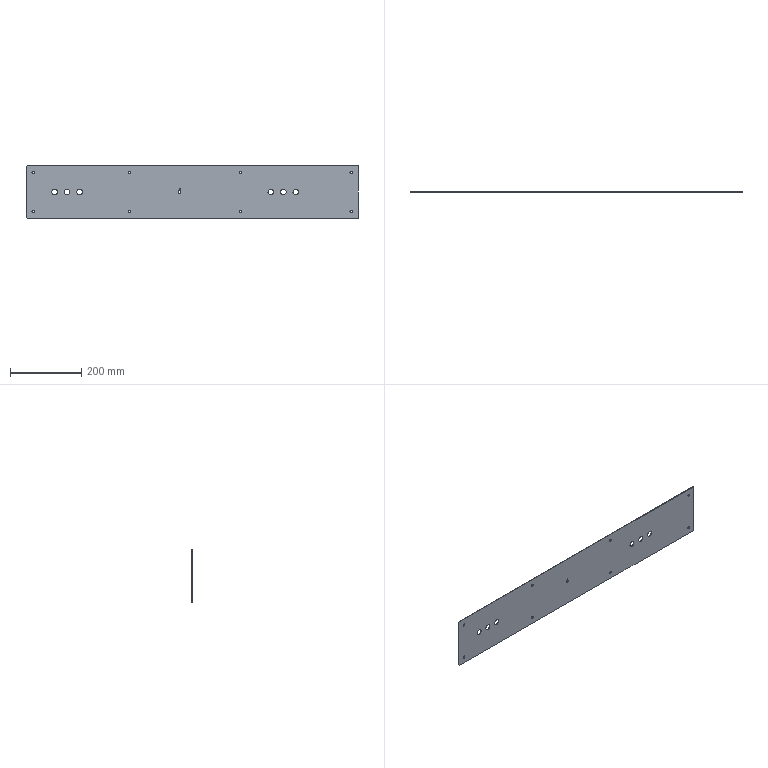Part | NX | 1 solid | 42 faces | box 929 x 2 x 150 mm | volume 275554 mm3 | cylinder 32 | plane 10 | commonest cylinder face diameters 7 x18 16 x12 3 x2
STEP:
#1=CARTESIAN_POINT('',(1280.5,-128.5,192.5));
#2=VERTEX_POINT('',#1);
#3=CARTESIAN_POINT('',(1287.5,-128.5,192.5));
#4=VERTEX_POINT('',#3);
#5=CARTESIAN_POINT('',(1284.,-128.5,192.5));
#6=DIRECTION('',(0.,-1.,0.));
#7=DIRECTION('',(1.,0.,0.));
#8=AXIS2_PLACEMENT_3D('',#5,#6,#7);
#9=CIRCLE('',#8,3.5);
#10=EDGE_CURVE('',#2,#4,#9,.T.);
#11=ORIENTED_EDGE('',*,*,#10,.T.);
#12=CARTESIAN_POINT('',(1287.5,-126.5,192.5));
#13=VERTEX_POINT('',#12);
#14=CARTESIAN_POINT('',(1287.5,-126.5,192.5));
#15=DIRECTION('',(0.,-1.,0.));
#16=VECTOR('',#15,1000.);
#17=LINE('',#14,#16);
#18=EDGE_CURVE('',#13,#4,#17,.T.);
#19=ORIENTED_EDGE('',*,*,#18,.F.);
#20=CARTESIAN_POINT('',(1280.5,-126.5,192.5));
#21=VERTEX_POINT('',#20);
#22=CARTESIAN_POINT('',(1284.,-126.5,192.5));
#23=DIRECTION('',(0.,-1.,0.));
#24=DIRECTION('',(1.,0.,0.));
#25=AXIS2_PLACEMENT_3D('',#22,#23,#24);
#26=CIRCLE('',#25,3.5);
#27=EDGE_CURVE('',#21,#13,#26,.T.);
#28=ORIENTED_EDGE('',*,*,#27,.F.);
#29=CARTESIAN_POINT('',(1280.5,-126.5,192.5));
#30=DIRECTION('',(0.,-1.,0.));
#31=VECTOR('',#30,1000.);
#32=LINE('',#29,#31);
#33=EDGE_CURVE('',#21,#2,#32,.T.);
#34=ORIENTED_EDGE('',*,*,#33,.T.);
#35=EDGE_LOOP('',(#11,#19,#28,#34));
#36=FACE_BOUND('',#35,.T.);
#37=CARTESIAN_POINT('',(1284.,-126.5,192.5));
#38=DIRECTION('',(0.,-1.,0.));
#39=DIRECTION('',(1.,0.,0.));
#40=AXIS2_PLACEMENT_3D('',#37,#38,#39);
#41=CYLINDRICAL_SURFACE('',#40,3.5);
#42=ADVANCED_FACE('',(#36),#41,.F.);
#43=ORIENTED_EDGE('',*,*,#18,.T.);
#44=CARTESIAN_POINT('',(1284.,-128.5,192.5));
#45=DIRECTION('',(0.,-1.,0.));
#46=DIRECTION('',(1.,0.,0.));
#47=AXIS2_PLACEMENT_3D('',#44,#45,#46);
#48=CIRCLE('',#47,3.5);
#49=EDGE_CURVE('',#4,#2,#48,.T.);
#50=ORIENTED_EDGE('',*,*,#49,.T.);
#51=ORIENTED_EDGE('',*,*,#33,.F.);
#52=CARTESIAN_POINT('',(1284.,-126.5,192.5));
#53=DIRECTION('',(0.,-1.,0.));
#54=DIRECTION('',(1.,0.,0.));
#55=AXIS2_PLACEMENT_3D('',#52,#53,#54);
#56=CIRCLE('',#55,3.5);
#57=EDGE_CURVE('',#13,#21,#56,.T.);
#58=ORIENTED_EDGE('',*,*,#57,.F.);
#59=EDGE_LOOP('',(#43,#50,#51,#58));
#60=FACE_BOUND('',#59,.T.);
#61=CARTESIAN_POINT('',(1284.,-126.5,192.5));
#62=DIRECTION('',(0.,-1.,0.));
#63=DIRECTION('',(1.,0.,0.));
#64=AXIS2_PLACEMENT_3D('',#61,#62,#63);
#65=CYLINDRICAL_SURFACE('',#64,3.5);
#66=ADVANCED_FACE('',(#60),#65,.F.);
#67=CARTESIAN_POINT('',(1757.,-128.5,137.5));
#68=VERTEX_POINT('',#67);
#69=CARTESIAN_POINT('',(1741.,-128.5,137.5));
#70=VERTEX_POINT('',#69);
#71=CARTESIAN_POINT('',(1749.,-128.5,137.5));
#72=DIRECTION('',(0.,-1.,0.));
#73=DIRECTION('',(1.,0.,0.));
#74=AXIS2_PLACEMENT_3D('',#71,#72,#73);
#75=CIRCLE('',#74,8.);
#76=EDGE_CURVE('',#68,#70,#75,.T.);
#77=ORIENTED_EDGE('',*,*,#76,.T.);
#78=CARTESIAN_POINT('',(1741.,-126.5,137.5));
#79=VERTEX_POINT('',#78);
#80=CARTESIAN_POINT('',(1741.,-126.5,137.5));
#81=DIRECTION('',(0.,-1.,0.));
#82=VECTOR('',#81,1000.);
#83=LINE('',#80,#82);
#84=EDGE_CURVE('',#79,#70,#83,.T.);
#85=ORIENTED_EDGE('',*,*,#84,.F.);
#86=CARTESIAN_POINT('',(1757.,-126.5,137.5));
#87=VERTEX_POINT('',#86);
#88=CARTESIAN_POINT('',(1749.,-126.5,137.5));
#89=DIRECTION('',(0.,-1.,0.));
#90=DIRECTION('',(1.,0.,0.));
#91=AXIS2_PLACEMENT_3D('',#88,#89,#90);
#92=CIRCLE('',#91,8.);
#93=EDGE_CURVE('',#87,#79,#92,.T.);
#94=ORIENTED_EDGE('',*,*,#93,.F.);
#95=CARTESIAN_POINT('',(1757.,-126.5,137.5));
#96=DIRECTION('',(0.,-1.,0.));
#97=VECTOR('',#96,1000.);
#98=LINE('',#95,#97);
#99=EDGE_CURVE('',#87,#68,#98,.T.);
#100=ORIENTED_EDGE('',*,*,#99,.T.);
#101=EDGE_LOOP('',(#77,#85,#94,#100));
#102=FACE_BOUND('',#101,.T.);
#103=CARTESIAN_POINT('',(1749.,-126.5,137.5));
#104=DIRECTION('',(0.,-1.,0.));
#105=DIRECTION('',(1.,0.,0.));
#106=AXIS2_PLACEMENT_3D('',#103,#104,#105);
#107=CYLINDRICAL_SURFACE('',#106,8.);
#108=ADVANCED_FACE('',(#102),#107,.F.);
#109=ORIENTED_EDGE('',*,*,#99,.F.);
#110=CARTESIAN_POINT('',(1749.,-126.5,137.5));
#111=DIRECTION('',(0.,-1.,0.));
#112=DIRECTION('',(1.,0.,0.));
#113=AXIS2_PLACEMENT_3D('',#110,#111,#112);
#114=CIRCLE('',#113,8.);
#115=EDGE_CURVE('',#79,#87,#114,.T.);
#116=ORIENTED_EDGE('',*,*,#115,.F.);
#117=ORIENTED_EDGE('',*,*,#84,.T.);
#118=CARTESIAN_POINT('',(1749.,-128.5,137.5));
#119=DIRECTION('',(0.,-1.,0.));
#120=DIRECTION('',(1.,0.,0.));
#121=AXIS2_PLACEMENT_3D('',#118,#119,#120);
#122=CIRCLE('',#121,8.);
#123=EDGE_CURVE('',#70,#68,#122,.T.);
#124=ORIENTED_EDGE('',*,*,#123,.T.);
#125=EDGE_LOOP('',(#109,#116,#117,#124));
#126=FACE_BOUND('',#125,.T.);
#127=CARTESIAN_POINT('',(1749.,-126.5,137.5));
#128=DIRECTION('',(0.,-1.,0.));
#129=DIRECTION('',(1.,0.,0.));
#130=AXIS2_PLACEMENT_3D('',#127,#128,#129);
#131=CYLINDRICAL_SURFACE('',#130,8.);
#132=ADVANCED_FACE('',(#126),#131,.F.);
#133=CARTESIAN_POINT('',(1923.,-126.5,64.5));
#134=VERTEX_POINT('',#133);
#135=CARTESIAN_POINT('',(1921.,-126.5,62.5));
#136=VERTEX_POINT('',#135);
#137=CARTESIAN_POINT('',(1769.238,-126.5,-89.262));
#138=DIRECTION('',(-0.7071,0.,-0.7071));
#139=VECTOR('',#138,1000.);
#140=LINE('',#137,#139);
#141=EDGE_CURVE('',#134,#136,#140,.T.);
#142=ORIENTED_EDGE('',*,*,#141,.F.);
#143=CARTESIAN_POINT('',(1923.,-128.5,64.5));
#144=VERTEX_POINT('',#143);
#145=CARTESIAN_POINT('',(1923.,278.,64.5));
#146=DIRECTION('',(0.,-1.,0.));
#147=VECTOR('',#146,1000.);
#148=LINE('',#145,#147);
#149=EDGE_CURVE('',#134,#144,#148,.T.);
#150=ORIENTED_EDGE('',*,*,#149,.T.);
#151=CARTESIAN_POINT('',(1921.,-128.5,62.5));
#152=VERTEX_POINT('',#151);
#153=CARTESIAN_POINT('',(1769.238,-128.5,-89.262));
#154=DIRECTION('',(-0.7071,0.,-0.7071));
#155=VECTOR('',#154,1000.);
#156=LINE('',#153,#155);
#157=EDGE_CURVE('',#144,#152,#156,.T.);
#158=ORIENTED_EDGE('',*,*,#157,.T.);
#159=CARTESIAN_POINT('',(1921.,-126.5,62.5));
#160=DIRECTION('',(0.,-1.,0.));
#161=VECTOR('',#160,1000.);
#162=LINE('',#159,#161);
#163=EDGE_CURVE('',#136,#152,#162,.T.);
#164=ORIENTED_EDGE('',*,*,#163,.F.);
#165=EDGE_LOOP('',(#142,#150,#158,#164));
#166=FACE_BOUND('',#165,.T.);
#167=CARTESIAN_POINT('',(1924.,-126.5,65.5));
#168=DIRECTION('',(0.7071,0.,-0.7071));
#169=DIRECTION('',(0.,-1.,0.));
#170=AXIS2_PLACEMENT_3D('',#167,#168,#169);
#171=PLANE('',#170);
#172=ADVANCED_FACE('',(#166),#171,.T.);
#173=CARTESIAN_POINT('',(1923.,-126.5,210.5));
#174=VERTEX_POINT('',#173);
#175=CARTESIAN_POINT('',(1923.,-126.5,-89.262));
#176=DIRECTION('',(0.,0.,1.));
#177=VECTOR('',#176,1000.);
#178=LINE('',#175,#177);
#179=EDGE_CURVE('',#134,#174,#178,.T.);
#180=ORIENTED_EDGE('',*,*,#179,.T.);
#181=CARTESIAN_POINT('',(1923.,-128.5,210.5));
#182=VERTEX_POINT('',#181);
#183=CARTESIAN_POINT('',(1923.,278.,210.5));
#184=DIRECTION('',(0.,1.,0.));
#185=VECTOR('',#184,1000.);
#186=LINE('',#183,#185);
#187=EDGE_CURVE('',#182,#174,#186,.T.);
#188=ORIENTED_EDGE('',*,*,#187,.F.);
#189=CARTESIAN_POINT('',(1923.,-128.5,-89.262));
#190=DIRECTION('',(0.,0.,1.));
#191=VECTOR('',#190,1000.);
#192=LINE('',#189,#191);
#193=EDGE_CURVE('',#144,#182,#192,.T.);
#194=ORIENTED_EDGE('',*,*,#193,.F.);
#195=ORIENTED_EDGE('',*,*,#149,.F.);
#196=EDGE_LOOP('',(#180,#188,#194,#195));
#197=FACE_BOUND('',#196,.T.);
#198=CARTESIAN_POINT('',(1923.,-126.5,209.5));
#199=DIRECTION('',(1.,0.,0.));
#200=DIRECTION('',(0.,1.,0.));
#201=AXIS2_PLACEMENT_3D('',#198,#199,#200);
#202=PLANE('',#201);
#203=ADVANCED_FACE('',(#197),#202,.T.);
#204=CARTESIAN_POINT('',(1921.,-126.5,212.5));
#205=VERTEX_POINT('',#204);
#206=CARTESIAN_POINT('',(2222.762,-126.5,-89.262));
#207=DIRECTION('',(0.7071,0.,-0.7071));
#208=VECTOR('',#207,1000.);
#209=LINE('',#206,#208);
#210=EDGE_CURVE('',#205,#174,#209,.T.);
#211=ORIENTED_EDGE('',*,*,#210,.F.);
#212=CARTESIAN_POINT('',(1921.,-128.5,212.5));
#213=VERTEX_POINT('',#212);
#214=CARTESIAN_POINT('',(1921.,-126.5,212.5));
#215=DIRECTION('',(0.,-1.,0.));
#216=VECTOR('',#215,1000.);
#217=LINE('',#214,#216);
#218=EDGE_CURVE('',#205,#213,#217,.T.);
#219=ORIENTED_EDGE('',*,*,#218,.T.);
#220=CARTESIAN_POINT('',(2222.762,-128.5,-89.262));
#221=DIRECTION('',(0.7071,0.,-0.7071));
#222=VECTOR('',#221,1000.);
#223=LINE('',#220,#222);
#224=EDGE_CURVE('',#213,#182,#223,.T.);
#225=ORIENTED_EDGE('',*,*,#224,.T.);
#226=ORIENTED_EDGE('',*,*,#187,.T.);
#227=EDGE_LOOP('',(#211,#219,#225,#226));
#228=FACE_BOUND('',#227,.T.);
#229=CARTESIAN_POINT('',(1921.,-126.5,212.5));
#230=DIRECTION('',(0.7071,0.,0.7071));
#231=DIRECTION('',(0.,-1.,0.));
#232=AXIS2_PLACEMENT_3D('',#229,#230,#231);
#233=PLANE('',#232);
#234=ADVANCED_FACE('',(#228),#233,.T.);
#235=CARTESIAN_POINT('',(997.,-126.5,212.5));
#236=VERTEX_POINT('',#235);
#237=CARTESIAN_POINT('',(1921.,-126.5,212.5));
#238=DIRECTION('',(-1.,0.,0.));
#239=VECTOR('',#238,1000.);
#240=LINE('',#237,#239);
#241=EDGE_CURVE('',#205,#236,#240,.T.);
#242=ORIENTED_EDGE('',*,*,#241,.T.);
#243=CARTESIAN_POINT('',(997.,-128.5,212.5));
#244=VERTEX_POINT('',#243);
#245=CARTESIAN_POINT('',(997.,-126.5,212.5));
#246=DIRECTION('',(0.,-1.,0.));
#247=VECTOR('',#246,1000.);
#248=LINE('',#245,#247);
#249=EDGE_CURVE('',#236,#244,#248,.T.);
#250=ORIENTED_EDGE('',*,*,#249,.T.);
#251=CARTESIAN_POINT('',(1921.,-128.5,212.5));
#252=DIRECTION('',(-1.,0.,0.));
#253=VECTOR('',#252,1000.);
#254=LINE('',#251,#253);
#255=EDGE_CURVE('',#213,#244,#254,.T.);
#256=ORIENTED_EDGE('',*,*,#255,.F.);
#257=ORIENTED_EDGE('',*,*,#218,.F.);
#258=EDGE_LOOP('',(#242,#250,#256,#257));
#259=FACE_BOUND('',#258,.T.);
#260=CARTESIAN_POINT('',(997.,-126.5,212.5));
#261=DIRECTION('',(0.,0.,1.));
#262=DIRECTION('',(1.,0.,0.));
#263=AXIS2_PLACEMENT_3D('',#260,#261,#262);
#264=PLANE('',#263);
#265=ADVANCED_FACE('',(#259),#264,.T.);
#266=CARTESIAN_POINT('',(994.,-126.5,209.5));
#267=VERTEX_POINT('',#266);
#268=CARTESIAN_POINT('',(994.,-126.5,209.5));
#269=DIRECTION('',(0.7071,0.,0.7071));
#270=VECTOR('',#269,1000.);
#271=LINE('',#268,#270);
#272=EDGE_CURVE('',#267,#236,#271,.T.);
#273=ORIENTED_EDGE('',*,*,#272,.F.);
#274=CARTESIAN_POINT('',(994.,-128.5,209.5));
#275=VERTEX_POINT('',#274);
#276=CARTESIAN_POINT('',(994.,-126.5,209.5));
#277=DIRECTION('',(0.,-1.,0.));
#278=VECTOR('',#277,1000.);
#279=LINE('',#276,#278);
#280=EDGE_CURVE('',#267,#275,#279,.T.);
#281=ORIENTED_EDGE('',*,*,#280,.T.);
#282=CARTESIAN_POINT('',(994.,-128.5,209.5));
#283=DIRECTION('',(0.7071,0.,0.7071));
#284=VECTOR('',#283,1000.);
#285=LINE('',#282,#284);
#286=EDGE_CURVE('',#275,#244,#285,.T.);
#287=ORIENTED_EDGE('',*,*,#286,.T.);
#288=ORIENTED_EDGE('',*,*,#249,.F.);
#289=EDGE_LOOP('',(#273,#281,#287,#288));
#290=FACE_BOUND('',#289,.T.);
#291=CARTESIAN_POINT('',(994.,-126.5,209.5));
#292=DIRECTION('',(-0.7071,0.,0.7071));
#293=DIRECTION('',(0.,1.,0.));
#294=AXIS2_PLACEMENT_3D('',#291,#292,#293);
#295=PLANE('',#294);
#296=ADVANCED_FACE('',(#290),#295,.T.);
#297=CARTESIAN_POINT('',(994.,-126.5,65.5));
#298=VERTEX_POINT('',#297);
#299=CARTESIAN_POINT('',(994.,-126.5,65.5));
#300=DIRECTION('',(0.,0.,1.));
#301=VECTOR('',#300,1000.);
#302=LINE('',#299,#301);
#303=EDGE_CURVE('',#298,#267,#302,.T.);
#304=ORIENTED_EDGE('',*,*,#303,.F.);
#305=CARTESIAN_POINT('',(994.,-128.5,65.5));
#306=VERTEX_POINT('',#305);
#307=CARTESIAN_POINT('',(994.,-126.5,65.5));
#308=DIRECTION('',(0.,-1.,0.));
#309=VECTOR('',#308,1000.);
#310=LINE('',#307,#309);
#311=EDGE_CURVE('',#298,#306,#310,.T.);
#312=ORIENTED_EDGE('',*,*,#311,.T.);
#313=CARTESIAN_POINT('',(994.,-128.5,65.5));
#314=DIRECTION('',(0.,0.,1.));
#315=VECTOR('',#314,1000.);
#316=LINE('',#313,#315);
#317=EDGE_CURVE('',#306,#275,#316,.T.);
#318=ORIENTED_EDGE('',*,*,#317,.T.);
#319=ORIENTED_EDGE('',*,*,#280,.F.);
#320=EDGE_LOOP('',(#304,#312,#318,#319));
#321=FACE_BOUND('',#320,.T.);
#322=CARTESIAN_POINT('',(994.,-126.5,65.5));
#323=DIRECTION('',(-1.,0.,0.));
#324=DIRECTION('',(0.,0.,1.));
#325=AXIS2_PLACEMENT_3D('',#322,#323,#324);
#326=PLANE('',#325);
#327=ADVANCED_FACE('',(#321),#326,.T.);
#328=CARTESIAN_POINT('',(997.,-126.5,62.5));
#329=VERTEX_POINT('',#328);
#330=CARTESIAN_POINT('',(997.,-126.5,62.5));
#331=DIRECTION('',(-0.7071,0.,0.7071));
#332=VECTOR('',#331,1000.);
#333=LINE('',#330,#332);
#334=EDGE_CURVE('',#329,#298,#333,.T.);
#335=ORIENTED_EDGE('',*,*,#334,.F.);
#336=CARTESIAN_POINT('',(997.,-128.5,62.5));
#337=VERTEX_POINT('',#336);
#338=CARTESIAN_POINT('',(997.,-126.5,62.5));
#339=DIRECTION('',(0.,-1.,0.));
#340=VECTOR('',#339,1000.);
#341=LINE('',#338,#340);
#342=EDGE_CURVE('',#329,#337,#341,.T.);
#343=ORIENTED_EDGE('',*,*,#342,.T.);
#344=CARTESIAN_POINT('',(997.,-128.5,62.5));
#345=DIRECTION('',(-0.7071,0.,0.7071));
#346=VECTOR('',#345,1000.);
#347=LINE('',#344,#346);
#348=EDGE_CURVE('',#337,#306,#347,.T.);
#349=ORIENTED_EDGE('',*,*,#348,.T.);
#350=ORIENTED_EDGE('',*,*,#311,.F.);
#351=EDGE_LOOP('',(#335,#343,#349,#350));
#352=FACE_BOUND('',#351,.T.);
#353=CARTESIAN_POINT('',(997.,-126.5,62.5));
#354=DIRECTION('',(-0.7071,0.,-0.7071));
#355=DIRECTION('',(-0.7071,0.,0.7071));
#356=AXIS2_PLACEMENT_3D('',#353,#354,#355);
#357=PLANE('',#356);
#358=ADVANCED_FACE('',(#352),#357,.T.);
#359=CARTESIAN_POINT('',(997.,-126.5,62.5));
#360=DIRECTION('',(1.,0.,0.));
#361=VECTOR('',#360,1000.);
#362=LINE('',#359,#361);
#363=EDGE_CURVE('',#329,#136,#362,.T.);
#364=ORIENTED_EDGE('',*,*,#363,.T.);
#365=ORIENTED_EDGE('',*,*,#163,.T.);
#366=CARTESIAN_POINT('',(997.,-128.5,62.5));
#367=DIRECTION('',(1.,0.,0.));
#368=VECTOR('',#367,1000.);
#369=LINE('',#366,#368);
#370=EDGE_CURVE('',#337,#152,#369,.T.);
#371=ORIENTED_EDGE('',*,*,#370,.F.);
#372=ORIENTED_EDGE('',*,*,#342,.F.);
#373=EDGE_LOOP('',(#364,#365,#371,#372));
#374=FACE_BOUND('',#373,.T.);
#375=CARTESIAN_POINT('',(1921.,-126.5,62.5));
#376=DIRECTION('',(0.,0.,-1.));
#377=DIRECTION('',(0.,-1.,0.));
#378=AXIS2_PLACEMENT_3D('',#375,#376,#377);
#379=PLANE('',#378);
#380=ADVANCED_FACE('',(#374),#379,.T.);
#381=CARTESIAN_POINT('',(1907.5,-128.5,192.5));
#382=VERTEX_POINT('',#381);
#383=CARTESIAN_POINT('',(1900.5,-128.5,192.5));
#384=VERTEX_POINT('',#383);
#385=CARTESIAN_POINT('',(1904.,-128.5,192.5));
#386=DIRECTION('',(0.,-1.,0.));
#387=DIRECTION('',(1.,0.,0.));
#388=AXIS2_PLACEMENT_3D('',#385,#386,#387);
#389=CIRCLE('',#388,3.5);
#390=EDGE_CURVE('',#382,#384,#389,.T.);
#391=ORIENTED_EDGE('',*,*,#390,.T.);
#392=CARTESIAN_POINT('',(1900.5,-126.5,192.5));
#393=VERTEX_POINT('',#392);
#394=CARTESIAN_POINT('',(1900.5,-126.5,192.5));
#395=DIRECTION('',(0.,-1.,0.));
#396=VECTOR('',#395,1000.);
#397=LINE('',#394,#396);
#398=EDGE_CURVE('',#393,#384,#397,.T.);
#399=ORIENTED_EDGE('',*,*,#398,.F.);
#400=CARTESIAN_POINT('',(1907.5,-126.5,192.5));
#401=VERTEX_POINT('',#400);
#402=CARTESIAN_POINT('',(1904.,-126.5,192.5));
#403=DIRECTION('',(0.,-1.,0.));
#404=DIRECTION('',(1.,0.,0.));
#405=AXIS2_PLACEMENT_3D('',#402,#403,#404);
#406=CIRCLE('',#405,3.5);
#407=EDGE_CURVE('',#401,#393,#406,.T.);
#408=ORIENTED_EDGE('',*,*,#407,.F.);
#409=CARTESIAN_POINT('',(1907.5,-126.5,192.5));
#410=DIRECTION('',(0.,-1.,0.));
#411=VECTOR('',#410,1000.);
#412=LINE('',#409,#411);
#413=EDGE_CURVE('',#401,#382,#412,.T.);
#414=ORIENTED_EDGE('',*,*,#413,.T.);
#415=EDGE_LOOP('',(#391,#399,#408,#414));
#416=FACE_BOUND('',#415,.T.);
#417=CARTESIAN_POINT('',(1904.,-126.5,192.5));
#418=DIRECTION('',(0.,-1.,0.));
#419=DIRECTION('',(1.,0.,0.));
#420=AXIS2_PLACEMENT_3D('',#417,#418,#419);
#421=CYLINDRICAL_SURFACE('',#420,3.5);
#422=ADVANCED_FACE('',(#416),#421,.F.);
#423=ORIENTED_EDGE('',*,*,#413,.F.);
#424=CARTESIAN_POINT('',(1904.,-126.5,192.5));
#425=DIRECTION('',(0.,-1.,0.));
#426=DIRECTION('',(1.,0.,0.));
#427=AXIS2_PLACEMENT_3D('',#424,#425,#426);
#428=CIRCLE('',#427,3.5);
#429=EDGE_CURVE('',#393,#401,#428,.T.);
#430=ORIENTED_EDGE('',*,*,#429,.F.);
#431=ORIENTED_EDGE('',*,*,#398,.T.);
#432=CARTESIAN_POINT('',(1904.,-128.5,192.5));
#433=DIRECTION('',(0.,-1.,0.));
#434=DIRECTION('',(1.,0.,0.));
#435=AXIS2_PLACEMENT_3D('',#432,#433,#434);
#436=CIRCLE('',#435,3.5);
#437=EDGE_CURVE('',#384,#382,#436,.T.);
#438=ORIENTED_EDGE('',*,*,#437,.T.);
#439=EDGE_LOOP('',(#423,#430,#431,#438));
#440=FACE_BOUND('',#439,.T.);
#441=CARTESIAN_POINT('',(1904.,-126.5,192.5));
#442=DIRECTION('',(0.,-1.,0.));
#443=DIRECTION('',(1.,0.,0.));
#444=AXIS2_PLACEMENT_3D('',#441,#442,#443);
#445=CYLINDRICAL_SURFACE('',#444,3.5);
#446=ADVANCED_FACE('',(#440),#445,.F.);
#447=CARTESIAN_POINT('',(1287.5,-128.5,82.5));
#448=VERTEX_POINT('',#447);
#449=CARTESIAN_POINT('',(1280.5,-128.5,82.5));
#450=VERTEX_POINT('',#449);
#451=CARTESIAN_POINT('',(1284.,-128.5,82.5));
#452=DIRECTION('',(0.,-1.,0.));
#453=DIRECTION('',(1.,0.,0.));
#454=AXIS2_PLACEMENT_3D('',#451,#452,#453);
#455=CIRCLE('',#454,3.5);
#456=EDGE_CURVE('',#448,#450,#455,.T.);
#457=ORIENTED_EDGE('',*,*,#456,.T.);
#458=CARTESIAN_POINT('',(1280.5,-126.5,82.5));
#459=VERTEX_POINT('',#458);
#460=CARTESIAN_POINT('',(1280.5,-126.5,82.5));
#461=DIRECTION('',(0.,-1.,0.));
#462=VECTOR('',#461,1000.);
#463=LINE('',#460,#462);
#464=EDGE_CURVE('',#459,#450,#463,.T.);
#465=ORIENTED_EDGE('',*,*,#464,.F.);
#466=CARTESIAN_POINT('',(1287.5,-126.5,82.5));
#467=VERTEX_POINT('',#466);
#468=CARTESIAN_POINT('',(1284.,-126.5,82.5));
#469=DIRECTION('',(0.,-1.,0.));
#470=DIRECTION('',(1.,0.,0.));
#471=AXIS2_PLACEMENT_3D('',#468,#469,#470);
#472=CIRCLE('',#471,3.5);
#473=EDGE_CURVE('',#467,#459,#472,.T.);
#474=ORIENTED_EDGE('',*,*,#473,.F.);
#475=CARTESIAN_POINT('',(1287.5,-126.5,82.5));
#476=DIRECTION('',(0.,-1.,0.));
#477=VECTOR('',#476,1000.);
#478=LINE('',#475,#477);
#479=EDGE_CURVE('',#467,#448,#478,.T.);
#480=ORIENTED_EDGE('',*,*,#479,.T.);
#481=EDGE_LOOP('',(#457,#465,#474,#480));
#482=FACE_BOUND('',#481,.T.);
#483=CARTESIAN_POINT('',(1284.,-126.5,82.5));
#484=DIRECTION('',(0.,-1.,0.));
#485=DIRECTION('',(1.,0.,0.));
#486=AXIS2_PLACEMENT_3D('',#483,#484,#485);
#487=CYLINDRICAL_SURFACE('',#486,3.5);
#488=ADVANCED_FACE('',(#482),#487,.F.);
#489=ORIENTED_EDGE('',*,*,#479,.F.);
#490=CARTESIAN_POINT('',(1284.,-126.5,82.5));
#491=DIRECTION('',(0.,-1.,0.));
#492=DIRECTION('',(1.,0.,0.));
#493=AXIS2_PLACEMENT_3D('',#490,#491,#492);
#494=CIRCLE('',#493,3.5);
#495=EDGE_CURVE('',#459,#467,#494,.T.);
#496=ORIENTED_EDGE('',*,*,#495,.F.);
#497=ORIENTED_EDGE('',*,*,#464,.T.);
#498=CARTESIAN_POINT('',(1284.,-128.5,82.5));
#499=DIRECTION('',(0.,-1.,0.));
#500=DIRECTION('',(1.,0.,0.));
#501=AXIS2_PLACEMENT_3D('',#498,#499,#500);
#502=CIRCLE('',#501,3.5);
#503=EDGE_CURVE('',#450,#448,#502,.T.);
#504=ORIENTED_EDGE('',*,*,#503,.T.);
#505=EDGE_LOOP('',(#489,#496,#497,#504));
#506=FACE_BOUND('',#505,.T.);
#507=CARTESIAN_POINT('',(1284.,-126.5,82.5));
#508=DIRECTION('',(0.,-1.,0.));
#509=DIRECTION('',(1.,0.,0.));
#510=AXIS2_PLACEMENT_3D('',#507,#508,#509);
#511=CYLINDRICAL_SURFACE('',#510,3.5);
#512=ADVANCED_FACE('',(#506),#511,.F.);
#513=CARTESIAN_POINT('',(1597.5,-128.5,82.5));
#514=VERTEX_POINT('',#513);
#515=CARTESIAN_POINT('',(1590.5,-128.5,82.5));
#516=VERTEX_POINT('',#515);
#517=CARTESIAN_POINT('',(1594.,-128.5,82.5));
#518=DIRECTION('',(0.,-1.,0.));
#519=DIRECTION('',(1.,0.,0.));
#520=AXIS2_PLACEMENT_3D('',#517,#518,#519);
#521=CIRCLE('',#520,3.5);
#522=EDGE_CURVE('',#514,#516,#521,.T.);
#523=ORIENTED_EDGE('',*,*,#522,.T.);
#524=CARTESIAN_POINT('',(1590.5,-126.5,82.5));
#525=VERTEX_POINT('',#524);
#526=CARTESIAN_POINT('',(1590.5,-126.5,82.5));
#527=DIRECTION('',(0.,-1.,0.));
#528=VECTOR('',#527,1000.);
#529=LINE('',#526,#528);
#530=EDGE_CURVE('',#525,#516,#529,.T.);
#531=ORIENTED_EDGE('',*,*,#530,.F.);
#532=CARTESIAN_POINT('',(1597.5,-126.5,82.5));
#533=VERTEX_POINT('',#532);
#534=CARTESIAN_POINT('',(1594.,-126.5,82.5));
#535=DIRECTION('',(0.,-1.,0.));
#536=DIRECTION('',(1.,0.,0.));
#537=AXIS2_PLACEMENT_3D('',#534,#535,#536);
#538=CIRCLE('',#537,3.5);
#539=EDGE_CURVE('',#533,#525,#538,.T.);
#540=ORIENTED_EDGE('',*,*,#539,.F.);
#541=CARTESIAN_POINT('',(1597.5,-126.5,82.5));
#542=DIRECTION('',(0.,-1.,0.));
#543=VECTOR('',#542,1000.);
#544=LINE('',#541,#543);
#545=EDGE_CURVE('',#533,#514,#544,.T.);
#546=ORIENTED_EDGE('',*,*,#545,.T.);
#547=EDGE_LOOP('',(#523,#531,#540,#546));
#548=FACE_BOUND('',#547,.T.);
#549=CARTESIAN_POINT('',(1594.,-126.5,82.5));
#550=DIRECTION('',(0.,-1.,0.));
#551=DIRECTION('',(1.,0.,0.));
#552=AXIS2_PLACEMENT_3D('',#549,#550,#551);
#553=CYLINDRICAL_SURFACE('',#552,3.5);
#554=ADVANCED_FACE('',(#548),#553,.F.);
#555=ORIENTED_EDGE('',*,*,#545,.F.);
#556=CARTESIAN_POINT('',(1594.,-126.5,82.5));
#557=DIRECTION('',(0.,-1.,0.));
#558=DIRECTION('',(1.,0.,0.));
#559=AXIS2_PLACEMENT_3D('',#556,#557,#558);
#560=CIRCLE('',#559,3.5);
#561=EDGE_CURVE('',#525,#533,#560,.T.);
#562=ORIENTED_EDGE('',*,*,#561,.F.);
#563=ORIENTED_EDGE('',*,*,#530,.T.);
#564=CARTESIAN_POINT('',(1594.,-128.5,82.5));
#565=DIRECTION('',(0.,-1.,0.));
#566=DIRECTION('',(1.,0.,0.));
#567=AXIS2_PLACEMENT_3D('',#564,#565,#566);
#568=CIRCLE('',#567,3.5);
#569=EDGE_CURVE('',#516,#514,#568,.T.);
#570=ORIENTED_EDGE('',*,*,#569,.T.);
#571=EDGE_LOOP('',(#555,#562,#563,#570));
#572=FACE_BOUND('',#571,.T.);
#573=CARTESIAN_POINT('',(1594.,-126.5,82.5));
#574=DIRECTION('',(0.,-1.,0.));
#575=DIRECTION('',(1.,0.,0.));
#576=AXIS2_PLACEMENT_3D('',#573,#574,#575);
#577=CYLINDRICAL_SURFACE('',#576,3.5);
#578=ADVANCED_FACE('',(#572),#577,.F.);
#579=CARTESIAN_POINT('',(1017.5,-128.5,82.5));
#580=VERTEX_POINT('',#579);
#581=CARTESIAN_POINT('',(1010.5,-128.5,82.5));
#582=VERTEX_POINT('',#581);
#583=CARTESIAN_POINT('',(1014.,-128.5,82.5));
#584=DIRECTION('',(0.,-1.,0.));
#585=DIRECTION('',(1.,0.,0.));
#586=AXIS2_PLACEMENT_3D('',#583,#584,#585);
#587=CIRCLE('',#586,3.5);
#588=EDGE_CURVE('',#580,#582,#587,.T.);
#589=ORIENTED_EDGE('',*,*,#588,.T.);
#590=CARTESIAN_POINT('',(1010.5,-126.5,82.5));
#591=VERTEX_POINT('',#590);
#592=CARTESIAN_POINT('',(1010.5,-126.5,82.5));
#593=DIRECTION('',(0.,-1.,0.));
#594=VECTOR('',#593,1000.);
#595=LINE('',#592,#594);
#596=EDGE_CURVE('',#591,#582,#595,.T.);
#597=ORIENTED_EDGE('',*,*,#596,.F.);
#598=CARTESIAN_POINT('',(1017.5,-126.5,82.5));
#599=VERTEX_POINT('',#598);
#600=CARTESIAN_POINT('',(1014.,-126.5,82.5));
#601=DIRECTION('',(0.,-1.,0.));
#602=DIRECTION('',(1.,0.,0.));
#603=AXIS2_PLACEMENT_3D('',#600,#601,#602);
#604=CIRCLE('',#603,3.5);
#605=EDGE_CURVE('',#599,#591,#604,.T.);
#606=ORIENTED_EDGE('',*,*,#605,.F.);
#607=CARTESIAN_POINT('',(1017.5,-126.5,82.5));
#608=DIRECTION('',(0.,-1.,0.));
#609=VECTOR('',#608,1000.);
#610=LINE('',#607,#609);
#611=EDGE_CURVE('',#599,#580,#610,.T.);
#612=ORIENTED_EDGE('',*,*,#611,.T.);
#613=EDGE_LOOP('',(#589,#597,#606,#612));
#614=FACE_BOUND('',#613,.T.);
#615=CARTESIAN_POINT('',(1014.,-126.5,82.5));
#616=DIRECTION('',(0.,-1.,0.));
#617=DIRECTION('',(1.,0.,0.));
#618=AXIS2_PLACEMENT_3D('',#615,#616,#617);
#619=CYLINDRICAL_SURFACE('',#618,3.5);
#620=ADVANCED_FACE('',(#614),#619,.F.);
#621=ORIENTED_EDGE('',*,*,#611,.F.);
#622=CARTESIAN_POINT('',(1014.,-126.5,82.5));
#623=DIRECTION('',(0.,-1.,0.));
#624=DIRECTION('',(1.,0.,0.));
#625=AXIS2_PLACEMENT_3D('',#622,#623,#624);
#626=CIRCLE('',#625,3.5);
#627=EDGE_CURVE('',#591,#599,#626,.T.);
#628=ORIENTED_EDGE('',*,*,#627,.F.);
#629=ORIENTED_EDGE('',*,*,#596,.T.);
#630=CARTESIAN_POINT('',(1014.,-128.5,82.5));
#631=DIRECTION('',(0.,-1.,0.));
#632=DIRECTION('',(1.,0.,0.));
#633=AXIS2_PLACEMENT_3D('',#630,#631,#632);
#634=CIRCLE('',#633,3.5);
#635=EDGE_CURVE('',#582,#580,#634,.T.);
#636=ORIENTED_EDGE('',*,*,#635,.T.);
#637=EDGE_LOOP('',(#621,#628,#629,#636));
#638=FACE_BOUND('',#637,.T.);
#639=CARTESIAN_POINT('',(1014.,-126.5,82.5));
#640=DIRECTION('',(0.,-1.,0.));
#641=DIRECTION('',(1.,0.,0.));
#642=AXIS2_PLACEMENT_3D('',#639,#640,#641);
#643=CYLINDRICAL_SURFACE('',#642,3.5);
#644=ADVANCED_FACE('',(#638),#643,.F.);
#645=CARTESIAN_POINT('',(1590.5,-128.5,192.5));
#646=VERTEX_POINT('',#645);
#647=CARTESIAN_POINT('',(1597.5,-128.5,192.5));
#648=VERTEX_POINT('',#647);
#649=CARTESIAN_POINT('',(1594.,-128.5,192.5));
#650=DIRECTION('',(0.,-1.,0.));
#651=DIRECTION('',(1.,0.,0.));
#652=AXIS2_PLACEMENT_3D('',#649,#650,#651);
#653=CIRCLE('',#652,3.5);
#654=EDGE_CURVE('',#646,#648,#653,.T.);
#655=ORIENTED_EDGE('',*,*,#654,.T.);
#656=CARTESIAN_POINT('',(1597.5,-126.5,192.5));
#657=VERTEX_POINT('',#656);
#658=CARTESIAN_POINT('',(1597.5,-126.5,192.5));
#659=DIRECTION('',(0.,-1.,0.));
#660=VECTOR('',#659,1000.);
#661=LINE('',#658,#660);
#662=EDGE_CURVE('',#657,#648,#661,.T.);
#663=ORIENTED_EDGE('',*,*,#662,.F.);
#664=CARTESIAN_POINT('',(1590.5,-126.5,192.5));
#665=VERTEX_POINT('',#664);
#666=CARTESIAN_POINT('',(1594.,-126.5,192.5));
#667=DIRECTION('',(0.,-1.,0.));
#668=DIRECTION('',(1.,0.,0.));
#669=AXIS2_PLACEMENT_3D('',#666,#667,#668);
#670=CIRCLE('',#669,3.5);
#671=EDGE_CURVE('',#665,#657,#670,.T.);
#672=ORIENTED_EDGE('',*,*,#671,.F.);
#673=CARTESIAN_POINT('',(1590.5,-126.5,192.5));
#674=DIRECTION('',(0.,-1.,0.));
#675=VECTOR('',#674,1000.);
#676=LINE('',#673,#675);
#677=EDGE_CURVE('',#665,#646,#676,.T.);
#678=ORIENTED_EDGE('',*,*,#677,.T.);
#679=EDGE_LOOP('',(#655,#663,#672,#678));
#680=FACE_BOUND('',#679,.T.);
#681=CARTESIAN_POINT('',(1594.,-126.5,192.5));
#682=DIRECTION('',(0.,-1.,0.));
#683=DIRECTION('',(1.,0.,0.));
#684=AXIS2_PLACEMENT_3D('',#681,#682,#683);
#685=CYLINDRICAL_SURFACE('',#684,3.5);
#686=ADVANCED_FACE('',(#680),#685,.F.);
#687=ORIENTED_EDGE('',*,*,#662,.T.);
#688=CARTESIAN_POINT('',(1594.,-128.5,192.5));
#689=DIRECTION('',(0.,-1.,0.));
#690=DIRECTION('',(1.,0.,0.));
#691=AXIS2_PLACEMENT_3D('',#688,#689,#690);
#692=CIRCLE('',#691,3.5);
#693=EDGE_CURVE('',#648,#646,#692,.T.);
#694=ORIENTED_EDGE('',*,*,#693,.T.);
#695=ORIENTED_EDGE('',*,*,#677,.F.);
#696=CARTESIAN_POINT('',(1594.,-126.5,192.5));
#697=DIRECTION('',(0.,-1.,0.));
#698=DIRECTION('',(1.,0.,0.));
#699=AXIS2_PLACEMENT_3D('',#696,#697,#698);
#700=CIRCLE('',#699,3.5);
#701=EDGE_CURVE('',#657,#665,#700,.T.);
#702=ORIENTED_EDGE('',*,*,#701,.F.);
#703=EDGE_LOOP('',(#687,#694,#695,#702));
#704=FACE_BOUND('',#703,.T.);
#705=CARTESIAN_POINT('',(1594.,-126.5,192.5));
#706=DIRECTION('',(0.,-1.,0.));
#707=DIRECTION('',(1.,0.,0.));
#708=AXIS2_PLACEMENT_3D('',#705,#706,#707);
#709=CYLINDRICAL_SURFACE('',#708,3.5);
#710=ADVANCED_FACE('',(#704),#709,.F.);
#711=CARTESIAN_POINT('',(1136.,-128.5,137.5));
#712=VERTEX_POINT('',#711);
#713=CARTESIAN_POINT('',(1152.,-128.5,137.5));
#714=VERTEX_POINT('',#713);
#715=CARTESIAN_POINT('',(1144.,-128.5,137.5));
#716=DIRECTION('',(0.,-1.,0.));
#717=DIRECTION('',(1.,0.,0.));
#718=AXIS2_PLACEMENT_3D('',#715,#716,#717);
#719=CIRCLE('',#718,8.);
#720=EDGE_CURVE('',#712,#714,#719,.T.);
#721=ORIENTED_EDGE('',*,*,#720,.T.);
#722=CARTESIAN_POINT('',(1152.,-126.5,137.5));
#723=VERTEX_POINT('',#722);
#724=CARTESIAN_POINT('',(1152.,-126.5,137.5));
#725=DIRECTION('',(0.,-1.,0.));
#726=VECTOR('',#725,1000.);
#727=LINE('',#724,#726);
#728=EDGE_CURVE('',#723,#714,#727,.T.);
#729=ORIENTED_EDGE('',*,*,#728,.F.);
#730=CARTESIAN_POINT('',(1136.,-126.5,137.5));
#731=VERTEX_POINT('',#730);
#732=CARTESIAN_POINT('',(1144.,-126.5,137.5));
#733=DIRECTION('',(0.,-1.,0.));
#734=DIRECTION('',(1.,0.,0.));
#735=AXIS2_PLACEMENT_3D('',#732,#733,#734);
#736=CIRCLE('',#735,8.);
#737=EDGE_CURVE('',#731,#723,#736,.T.);
#738=ORIENTED_EDGE('',*,*,#737,.F.);
#739=CARTESIAN_POINT('',(1136.,-126.5,137.5));
#740=DIRECTION('',(0.,-1.,0.));
#741=VECTOR('',#740,1000.);
#742=LINE('',#739,#741);
#743=EDGE_CURVE('',#731,#712,#742,.T.);
#744=ORIENTED_EDGE('',*,*,#743,.T.);
#745=EDGE_LOOP('',(#721,#729,#738,#744));
#746=FACE_BOUND('',#745,.T.);
#747=CARTESIAN_POINT('',(1144.,-126.5,137.5));
#748=DIRECTION('',(0.,-1.,0.));
#749=DIRECTION('',(1.,0.,0.));
#750=AXIS2_PLACEMENT_3D('',#747,#748,#749);
#751=CYLINDRICAL_SURFACE('',#750,8.);
#752=ADVANCED_FACE('',(#746),#751,.F.);
#753=ORIENTED_EDGE('',*,*,#728,.T.);
#754=CARTESIAN_POINT('',(1144.,-128.5,137.5));
#755=DIRECTION('',(0.,-1.,0.));
#756=DIRECTION('',(1.,0.,0.));
#757=AXIS2_PLACEMENT_3D('',#754,#755,#756);
#758=CIRCLE('',#757,8.);
#759=EDGE_CURVE('',#714,#712,#758,.T.);
#760=ORIENTED_EDGE('',*,*,#759,.T.);
#761=ORIENTED_EDGE('',*,*,#743,.F.);
#762=CARTESIAN_POINT('',(1144.,-126.5,137.5));
#763=DIRECTION('',(0.,-1.,0.));
#764=DIRECTION('',(1.,0.,0.));
#765=AXIS2_PLACEMENT_3D('',#762,#763,#764);
#766=CIRCLE('',#765,8.);
#767=EDGE_CURVE('',#723,#731,#766,.T.);
#768=ORIENTED_EDGE('',*,*,#767,.F.);
#769=EDGE_LOOP('',(#753,#760,#761,#768));
#770=FACE_BOUND('',#769,.T.);
#771=CARTESIAN_POINT('',(1144.,-126.5,137.5));
#772=DIRECTION('',(0.,-1.,0.));
#773=DIRECTION('',(1.,0.,0.));
#774=AXIS2_PLACEMENT_3D('',#771,#772,#773);
#775=CYLINDRICAL_SURFACE('',#774,8.);
#776=ADVANCED_FACE('',(#770),#775,.F.);
#777=CARTESIAN_POINT('',(1010.5,-128.5,192.5));
#778=VERTEX_POINT('',#777);
#779=CARTESIAN_POINT('',(1017.5,-128.5,192.5));
#780=VERTEX_POINT('',#779);
#781=CARTESIAN_POINT('',(1014.,-128.5,192.5));
#782=DIRECTION('',(0.,-1.,0.));
#783=DIRECTION('',(1.,0.,0.));
#784=AXIS2_PLACEMENT_3D('',#781,#782,#783);
#785=CIRCLE('',#784,3.5);
#786=EDGE_CURVE('',#778,#780,#785,.T.);
#787=ORIENTED_EDGE('',*,*,#786,.T.);
#788=CARTESIAN_POINT('',(1017.5,-126.5,192.5));
#789=VERTEX_POINT('',#788);
#790=CARTESIAN_POINT('',(1017.5,-126.5,192.5));
#791=DIRECTION('',(0.,-1.,0.));
#792=VECTOR('',#791,1000.);
#793=LINE('',#790,#792);
#794=EDGE_CURVE('',#789,#780,#793,.T.);
#795=ORIENTED_EDGE('',*,*,#794,.F.);
#796=CARTESIAN_POINT('',(1010.5,-126.5,192.5));
#797=VERTEX_POINT('',#796);
#798=CARTESIAN_POINT('',(1014.,-126.5,192.5));
#799=DIRECTION('',(0.,-1.,0.));
#800=DIRECTION('',(1.,0.,0.));
#801=AXIS2_PLACEMENT_3D('',#798,#799,#800);
#802=CIRCLE('',#801,3.5);
#803=EDGE_CURVE('',#797,#789,#802,.T.);
#804=ORIENTED_EDGE('',*,*,#803,.F.);
#805=CARTESIAN_POINT('',(1010.5,-126.5,192.5));
#806=DIRECTION('',(0.,-1.,0.));
#807=VECTOR('',#806,1000.);
#808=LINE('',#805,#807);
#809=EDGE_CURVE('',#797,#778,#808,.T.);
#810=ORIENTED_EDGE('',*,*,#809,.T.);
#811=EDGE_LOOP('',(#787,#795,#804,#810));
#812=FACE_BOUND('',#811,.T.);
#813=CARTESIAN_POINT('',(1014.,-126.5,192.5));
#814=DIRECTION('',(0.,-1.,0.));
#815=DIRECTION('',(1.,0.,0.));
#816=AXIS2_PLACEMENT_3D('',#813,#814,#815);
#817=CYLINDRICAL_SURFACE('',#816,3.5);
#818=ADVANCED_FACE('',(#812),#817,.F.);
#819=ORIENTED_EDGE('',*,*,#794,.T.);
#820=CARTESIAN_POINT('',(1014.,-128.5,192.5));
#821=DIRECTION('',(0.,-1.,0.));
#822=DIRECTION('',(1.,0.,0.));
#823=AXIS2_PLACEMENT_3D('',#820,#821,#822);
#824=CIRCLE('',#823,3.5);
#825=EDGE_CURVE('',#780,#778,#824,.T.);
#826=ORIENTED_EDGE('',*,*,#825,.T.);
#827=ORIENTED_EDGE('',*,*,#809,.F.);
#828=CARTESIAN_POINT('',(1014.,-126.5,192.5));
#829=DIRECTION('',(0.,-1.,0.));
#830=DIRECTION('',(1.,0.,0.));
#831=AXIS2_PLACEMENT_3D('',#828,#829,#830);
#832=CIRCLE('',#831,3.5);
#833=EDGE_CURVE('',#789,#797,#832,.T.);
#834=ORIENTED_EDGE('',*,*,#833,.F.);
#835=EDGE_LOOP('',(#819,#826,#827,#834));
#836=FACE_BOUND('',#835,.T.);
#837=CARTESIAN_POINT('',(1014.,-126.5,192.5));
#838=DIRECTION('',(0.,-1.,0.));
#839=DIRECTION('',(1.,0.,0.));
#840=AXIS2_PLACEMENT_3D('',#837,#838,#839);
#841=CYLINDRICAL_SURFACE('',#840,3.5);
#842=ADVANCED_FACE('',(#836),#841,.F.);
#843=CARTESIAN_POINT('',(1427.5,-128.5,137.5));
#844=VERTEX_POINT('',#843);
#845=CARTESIAN_POINT('',(1420.5,-128.5,137.5));
#846=VERTEX_POINT('',#845);
#847=CARTESIAN_POINT('',(1424.,-128.5,137.5));
#848=DIRECTION('',(0.,-1.,0.));
#849=DIRECTION('',(1.,0.,0.));
#850=AXIS2_PLACEMENT_3D('',#847,#848,#849);
#851=CIRCLE('',#850,3.5);
#852=EDGE_CURVE('',#844,#846,#851,.T.);
#853=ORIENTED_EDGE('',*,*,#852,.T.);
#854=CARTESIAN_POINT('',(1420.5,-126.5,137.5));
#855=VERTEX_POINT('',#854);
#856=CARTESIAN_POINT('',(1420.5,-126.5,137.5));
#857=DIRECTION('',(0.,-1.,0.));
#858=VECTOR('',#857,1000.);
#859=LINE('',#856,#858);
#860=EDGE_CURVE('',#855,#846,#859,.T.);
#861=ORIENTED_EDGE('',*,*,#860,.F.);
#862=CARTESIAN_POINT('',(1427.5,-126.5,137.5));
#863=VERTEX_POINT('',#862);
#864=CARTESIAN_POINT('',(1424.,-126.5,137.5));
#865=DIRECTION('',(0.,-1.,0.));
#866=DIRECTION('',(1.,0.,0.));
#867=AXIS2_PLACEMENT_3D('',#864,#865,#866);
#868=CIRCLE('',#867,3.5);
#869=EDGE_CURVE('',#863,#855,#868,.T.);
#870=ORIENTED_EDGE('',*,*,#869,.F.);
#871=CARTESIAN_POINT('',(1427.5,-126.5,137.5));
#872=DIRECTION('',(0.,-1.,0.));
#873=VECTOR('',#872,1000.);
#874=LINE('',#871,#873);
#875=EDGE_CURVE('',#863,#844,#874,.T.);
#876=ORIENTED_EDGE('',*,*,#875,.T.);
#877=EDGE_LOOP('',(#853,#861,#870,#876));
#878=FACE_BOUND('',#877,.T.);
#879=CARTESIAN_POINT('',(1424.,-126.5,137.5));
#880=DIRECTION('',(0.,-1.,0.));
#881=DIRECTION('',(1.,0.,0.));
#882=AXIS2_PLACEMENT_3D('',#879,#880,#881);
#883=CYLINDRICAL_SURFACE('',#882,3.5);
#884=ADVANCED_FACE('',(#878),#883,.F.);
#885=ORIENTED_EDGE('',*,*,#875,.F.);
#886=CARTESIAN_POINT('',(1424.,-126.5,137.5));
#887=DIRECTION('',(0.,-1.,0.));
#888=DIRECTION('',(1.,0.,0.));
#889=AXIS2_PLACEMENT_3D('',#886,#887,#888);
#890=CIRCLE('',#889,3.5);
#891=EDGE_CURVE('',#855,#863,#890,.T.);
#892=ORIENTED_EDGE('',*,*,#891,.F.);
#893=ORIENTED_EDGE('',*,*,#860,.T.);
#894=CARTESIAN_POINT('',(1424.,-128.5,137.5));
#895=DIRECTION('',(0.,-1.,0.));
#896=DIRECTION('',(1.,0.,0.));
#897=AXIS2_PLACEMENT_3D('',#894,#895,#896);
#898=CIRCLE('',#897,3.5);
#899=EDGE_CURVE('',#846,#844,#898,.T.);
#900=ORIENTED_EDGE('',*,*,#899,.T.);
#901=EDGE_LOOP('',(#885,#892,#893,#900));
#902=FACE_BOUND('',#901,.T.);
#903=CARTESIAN_POINT('',(1424.,-126.5,137.5));
#904=DIRECTION('',(0.,-1.,0.));
#905=DIRECTION('',(1.,0.,0.));
#906=AXIS2_PLACEMENT_3D('',#903,#904,#905);
#907=CYLINDRICAL_SURFACE('',#906,3.5);
#908=ADVANCED_FACE('',(#902),#907,.F.);
#909=CARTESIAN_POINT('',(1082.,-128.5,137.5));
#910=VERTEX_POINT('',#909);
#911=CARTESIAN_POINT('',(1066.,-128.5,137.5));
#912=VERTEX_POINT('',#911);
#913=CARTESIAN_POINT('',(1074.,-128.5,137.5));
#914=DIRECTION('',(0.,-1.,0.));
#915=DIRECTION('',(1.,0.,0.));
#916=AXIS2_PLACEMENT_3D('',#913,#914,#915);
#917=CIRCLE('',#916,8.);
#918=EDGE_CURVE('',#910,#912,#917,.T.);
#919=ORIENTED_EDGE('',*,*,#918,.T.);
#920=CARTESIAN_POINT('',(1066.,-126.5,137.5));
#921=VERTEX_POINT('',#920);
#922=CARTESIAN_POINT('',(1066.,-126.5,137.5));
#923=DIRECTION('',(0.,-1.,0.));
#924=VECTOR('',#923,1000.);
#925=LINE('',#922,#924);
#926=EDGE_CURVE('',#921,#912,#925,.T.);
#927=ORIENTED_EDGE('',*,*,#926,.F.);
#928=CARTESIAN_POINT('',(1082.,-126.5,137.5));
#929=VERTEX_POINT('',#928);
#930=CARTESIAN_POINT('',(1074.,-126.5,137.5));
#931=DIRECTION('',(0.,-1.,0.));
#932=DIRECTION('',(1.,0.,0.));
#933=AXIS2_PLACEMENT_3D('',#930,#931,#932);
#934=CIRCLE('',#933,8.);
#935=EDGE_CURVE('',#929,#921,#934,.T.);
#936=ORIENTED_EDGE('',*,*,#935,.F.);
#937=CARTESIAN_POINT('',(1082.,-126.5,137.5));
#938=DIRECTION('',(0.,-1.,0.));
#939=VECTOR('',#938,1000.);
#940=LINE('',#937,#939);
#941=EDGE_CURVE('',#929,#910,#940,.T.);
#942=ORIENTED_EDGE('',*,*,#941,.T.);
#943=EDGE_LOOP('',(#919,#927,#936,#942));
#944=FACE_BOUND('',#943,.T.);
#945=CARTESIAN_POINT('',(1074.,-126.5,137.5));
#946=DIRECTION('',(0.,-1.,0.));
#947=DIRECTION('',(1.,0.,0.));
#948=AXIS2_PLACEMENT_3D('',#945,#946,#947);
#949=CYLINDRICAL_SURFACE('',#948,8.);
#950=ADVANCED_FACE('',(#944),#949,.F.);
#951=ORIENTED_EDGE('',*,*,#941,.F.);
#952=CARTESIAN_POINT('',(1074.,-126.5,137.5));
#953=DIRECTION('',(0.,-1.,0.));
#954=DIRECTION('',(1.,0.,0.));
#955=AXIS2_PLACEMENT_3D('',#952,#953,#954);
#956=CIRCLE('',#955,8.);
#957=EDGE_CURVE('',#921,#929,#956,.T.);
#958=ORIENTED_EDGE('',*,*,#957,.F.);
#959=ORIENTED_EDGE('',*,*,#926,.T.);
#960=CARTESIAN_POINT('',(1074.,-128.5,137.5));
#961=DIRECTION('',(0.,-1.,0.));
#962=DIRECTION('',(1.,0.,0.));
#963=AXIS2_PLACEMENT_3D('',#960,#961,#962);
#964=CIRCLE('',#963,8.);
#965=EDGE_CURVE('',#912,#910,#964,.T.);
#966=ORIENTED_EDGE('',*,*,#965,.T.);
#967=EDGE_LOOP('',(#951,#958,#959,#966));
#968=FACE_BOUND('',#967,.T.);
#969=CARTESIAN_POINT('',(1074.,-126.5,137.5));
#970=DIRECTION('',(0.,-1.,0.));
#971=DIRECTION('',(1.,0.,0.));
#972=AXIS2_PLACEMENT_3D('',#969,#970,#971);
#973=CYLINDRICAL_SURFACE('',#972,8.);
#974=ADVANCED_FACE('',(#968),#973,.F.);
#975=CARTESIAN_POINT('',(1907.5,-128.5,82.5));
#976=VERTEX_POINT('',#975);
#977=CARTESIAN_POINT('',(1900.5,-128.5,82.5));
#978=VERTEX_POINT('',#977);
#979=CARTESIAN_POINT('',(1904.,-128.5,82.5));
#980=DIRECTION('',(0.,-1.,0.));
#981=DIRECTION('',(1.,0.,0.));
#982=AXIS2_PLACEMENT_3D('',#979,#980,#981);
#983=CIRCLE('',#982,3.5);
#984=EDGE_CURVE('',#976,#978,#983,.T.);
#985=ORIENTED_EDGE('',*,*,#984,.T.);
#986=CARTESIAN_POINT('',(1900.5,-126.5,82.5));
#987=VERTEX_POINT('',#986);
#988=CARTESIAN_POINT('',(1900.5,-126.5,82.5));
#989=DIRECTION('',(0.,-1.,0.));
#990=VECTOR('',#989,1000.);
#991=LINE('',#988,#990);
#992=EDGE_CURVE('',#987,#978,#991,.T.);
#993=ORIENTED_EDGE('',*,*,#992,.F.);
#994=CARTESIAN_POINT('',(1907.5,-126.5,82.5));
#995=VERTEX_POINT('',#994);
#996=CARTESIAN_POINT('',(1904.,-126.5,82.5));
#997=DIRECTION('',(0.,-1.,0.));
#998=DIRECTION('',(1.,0.,0.));
#999=AXIS2_PLACEMENT_3D('',#996,#997,#998);
#1000=CIRCLE('',#999,3.5);
#1001=EDGE_CURVE('',#995,#987,#1000,.T.);
#1002=ORIENTED_EDGE('',*,*,#1001,.F.);
#1003=CARTESIAN_POINT('',(1907.5,-126.5,82.5));
#1004=DIRECTION('',(0.,-1.,0.));
#1005=VECTOR('',#1004,1000.);
#1006=LINE('',#1003,#1005);
#1007=EDGE_CURVE('',#995,#976,#1006,.T.);
#1008=ORIENTED_EDGE('',*,*,#1007,.T.);
#1009=EDGE_LOOP('',(#985,#993,#1002,#1008));
#1010=FACE_BOUND('',#1009,.T.);
#1011=CARTESIAN_POINT('',(1904.,-126.5,82.5));
#1012=DIRECTION('',(0.,-1.,0.));
#1013=DIRECTION('',(1.,0.,0.));
#1014=AXIS2_PLACEMENT_3D('',#1011,#1012,#1013);
#1015=CYLINDRICAL_SURFACE('',#1014,3.5);
#1016=ADVANCED_FACE('',(#1010),#1015,.F.);
#1017=ORIENTED_EDGE('',*,*,#1007,.F.);
#1018=CARTESIAN_POINT('',(1904.,-126.5,82.5));
#1019=DIRECTION('',(0.,-1.,0.));
#1020=DIRECTION('',(1.,0.,0.));
#1021=AXIS2_PLACEMENT_3D('',#1018,#1019,#1020);
#1022=CIRCLE('',#1021,3.5);
#1023=EDGE_CURVE('',#987,#995,#1022,.T.);
#1024=ORIENTED_EDGE('',*,*,#1023,.F.);
#1025=ORIENTED_EDGE('',*,*,#992,.T.);
#1026=CARTESIAN_POINT('',(1904.,-128.5,82.5));
#1027=DIRECTION('',(0.,-1.,0.));
#1028=DIRECTION('',(1.,0.,0.));
#1029=AXIS2_PLACEMENT_3D('',#1026,#1027,#1028);
#1030=CIRCLE('',#1029,3.5);
#1031=EDGE_CURVE('',#978,#976,#1030,.T.);
#1032=ORIENTED_EDGE('',*,*,#1031,.T.);
#1033=EDGE_LOOP('',(#1017,#1024,#1025,#1032));
#1034=FACE_BOUND('',#1033,.T.);
#1035=CARTESIAN_POINT('',(1904.,-126.5,82.5));
#1036=DIRECTION('',(0.,-1.,0.));
#1037=DIRECTION('',(1.,0.,0.));
#1038=AXIS2_PLACEMENT_3D('',#1035,#1036,#1037);
#1039=CYLINDRICAL_SURFACE('',#1038,3.5);
#1040=ADVANCED_FACE('',(#1034),#1039,.F.);
#1041=CARTESIAN_POINT('',(1722.,-128.5,137.5));
#1042=VERTEX_POINT('',#1041);
#1043=CARTESIAN_POINT('',(1706.,-128.5,137.5));
#1044=VERTEX_POINT('',#1043);
#1045=CARTESIAN_POINT('',(1714.,-128.5,137.5));
#1046=DIRECTION('',(0.,-1.,0.));
#1047=DIRECTION('',(1.,0.,0.));
#1048=AXIS2_PLACEMENT_3D('',#1045,#1046,#1047);
#1049=CIRCLE('',#1048,8.);
#1050=EDGE_CURVE('',#1042,#1044,#1049,.T.);
#1051=ORIENTED_EDGE('',*,*,#1050,.T.);
#1052=CARTESIAN_POINT('',(1706.,-126.5,137.5));
#1053=VERTEX_POINT('',#1052);
#1054=CARTESIAN_POINT('',(1706.,-126.5,137.5));
#1055=DIRECTION('',(0.,-1.,0.));
#1056=VECTOR('',#1055,1000.);
#1057=LINE('',#1054,#1056);
#1058=EDGE_CURVE('',#1053,#1044,#1057,.T.);
#1059=ORIENTED_EDGE('',*,*,#1058,.F.);
#1060=CARTESIAN_POINT('',(1722.,-126.5,137.5));
#1061=VERTEX_POINT('',#1060);
#1062=CARTESIAN_POINT('',(1714.,-126.5,137.5));
#1063=DIRECTION('',(0.,-1.,0.));
#1064=DIRECTION('',(1.,0.,0.));
#1065=AXIS2_PLACEMENT_3D('',#1062,#1063,#1064);
#1066=CIRCLE('',#1065,8.);
#1067=EDGE_CURVE('',#1061,#1053,#1066,.T.);
#1068=ORIENTED_EDGE('',*,*,#1067,.F.);
#1069=CARTESIAN_POINT('',(1722.,-126.5,137.5));
#1070=DIRECTION('',(0.,-1.,0.));
#1071=VECTOR('',#1070,1000.);
#1072=LINE('',#1069,#1071);
#1073=EDGE_CURVE('',#1061,#1042,#1072,.T.);
#1074=ORIENTED_EDGE('',*,*,#1073,.T.);
#1075=EDGE_LOOP('',(#1051,#1059,#1068,#1074));
#1076=FACE_BOUND('',#1075,.T.);
#1077=CARTESIAN_POINT('',(1714.,-126.5,137.5));
#1078=DIRECTION('',(0.,-1.,0.));
#1079=DIRECTION('',(1.,0.,0.));
#1080=AXIS2_PLACEMENT_3D('',#1077,#1078,#1079);
#1081=CYLINDRICAL_SURFACE('',#1080,8.);
#1082=ADVANCED_FACE('',(#1076),#1081,.F.);
#1083=ORIENTED_EDGE('',*,*,#1073,.F.);
#1084=CARTESIAN_POINT('',(1714.,-126.5,137.5));
#1085=DIRECTION('',(0.,-1.,0.));
#1086=DIRECTION('',(1.,0.,0.));
#1087=AXIS2_PLACEMENT_3D('',#1084,#1085,#1086);
#1088=CIRCLE('',#1087,8.);
#1089=EDGE_CURVE('',#1053,#1061,#1088,.T.);
#1090=ORIENTED_EDGE('',*,*,#1089,.F.);
#1091=ORIENTED_EDGE('',*,*,#1058,.T.);
#1092=CARTESIAN_POINT('',(1714.,-128.5,137.5));
#1093=DIRECTION('',(0.,-1.,0.));
#1094=DIRECTION('',(1.,0.,0.));
#1095=AXIS2_PLACEMENT_3D('',#1092,#1093,#1094);
#1096=CIRCLE('',#1095,8.);
#1097=EDGE_CURVE('',#1044,#1042,#1096,.T.);
#1098=ORIENTED_EDGE('',*,*,#1097,.T.);
#1099=EDGE_LOOP('',(#1083,#1090,#1091,#1098));
#1100=FACE_BOUND('',#1099,.T.);
#1101=CARTESIAN_POINT('',(1714.,-126.5,137.5));
#1102=DIRECTION('',(0.,-1.,0.));
#1103=DIRECTION('',(1.,0.,0.));
#1104=AXIS2_PLACEMENT_3D('',#1101,#1102,#1103);
#1105=CYLINDRICAL_SURFACE('',#1104,8.);
#1106=ADVANCED_FACE('',(#1100),#1105,.F.);
#1107=CARTESIAN_POINT('',(1425.5,-126.5,145.9));
#1108=VERTEX_POINT('',#1107);
#1109=CARTESIAN_POINT('',(1422.5,-126.5,145.9));
#1110=VERTEX_POINT('',#1109);
#1111=CARTESIAN_POINT('',(1424.,-126.5,145.9));
#1112=DIRECTION('',(0.,-1.,0.));
#1113=DIRECTION('',(1.,0.,0.));
#1114=AXIS2_PLACEMENT_3D('',#1111,#1112,#1113);
#1115=CIRCLE('',#1114,1.5);
#1116=EDGE_CURVE('',#1108,#1110,#1115,.T.);
#1117=ORIENTED_EDGE('',*,*,#1116,.F.);
#1118=CARTESIAN_POINT('',(1425.5,-128.5,145.9));
#1119=VERTEX_POINT('',#1118);
#1120=CARTESIAN_POINT('',(1425.5,-126.5,145.9));
#1121=DIRECTION('',(0.,-1.,0.));
#1122=VECTOR('',#1121,1000.);
#1123=LINE('',#1120,#1122);
#1124=EDGE_CURVE('',#1108,#1119,#1123,.T.);
#1125=ORIENTED_EDGE('',*,*,#1124,.T.);
#1126=CARTESIAN_POINT('',(1422.5,-128.5,145.9));
#1127=VERTEX_POINT('',#1126);
#1128=CARTESIAN_POINT('',(1424.,-128.5,145.9));
#1129=DIRECTION('',(0.,-1.,0.));
#1130=DIRECTION('',(1.,0.,0.));
#1131=AXIS2_PLACEMENT_3D('',#1128,#1129,#1130);
#1132=CIRCLE('',#1131,1.5);
#1133=EDGE_CURVE('',#1119,#1127,#1132,.T.);
#1134=ORIENTED_EDGE('',*,*,#1133,.T.);
#1135=CARTESIAN_POINT('',(1422.5,-126.5,145.9));
#1136=DIRECTION('',(0.,-1.,0.));
#1137=VECTOR('',#1136,1000.);
#1138=LINE('',#1135,#1137);
#1139=EDGE_CURVE('',#1110,#1127,#1138,.T.);
#1140=ORIENTED_EDGE('',*,*,#1139,.F.);
#1141=EDGE_LOOP('',(#1117,#1125,#1134,#1140));
#1142=FACE_BOUND('',#1141,.T.);
#1143=CARTESIAN_POINT('',(1424.,-126.5,145.9));
#1144=DIRECTION('',(0.,-1.,0.));
#1145=DIRECTION('',(1.,0.,0.));
#1146=AXIS2_PLACEMENT_3D('',#1143,#1144,#1145);
#1147=CYLINDRICAL_SURFACE('',#1146,1.5);
#1148=ADVANCED_FACE('',(#1142),#1147,.F.);
#1149=CARTESIAN_POINT('',(1424.,-128.5,145.9));
#1150=DIRECTION('',(0.,-1.,0.));
#1151=DIRECTION('',(1.,0.,0.));
#1152=AXIS2_PLACEMENT_3D('',#1149,#1150,#1151);
#1153=CIRCLE('',#1152,1.5);
#1154=EDGE_CURVE('',#1127,#1119,#1153,.T.);
#1155=ORIENTED_EDGE('',*,*,#1154,.T.);
#1156=ORIENTED_EDGE('',*,*,#1124,.F.);
#1157=CARTESIAN_POINT('',(1424.,-126.5,145.9));
#1158=DIRECTION('',(0.,-1.,0.));
#1159=DIRECTION('',(1.,0.,0.));
#1160=AXIS2_PLACEMENT_3D('',#1157,#1158,#1159);
#1161=CIRCLE('',#1160,1.5);
#1162=EDGE_CURVE('',#1110,#1108,#1161,.T.);
#1163=ORIENTED_EDGE('',*,*,#1162,.F.);
#1164=ORIENTED_EDGE('',*,*,#1139,.T.);
#1165=EDGE_LOOP('',(#1155,#1156,#1163,#1164));
#1166=FACE_BOUND('',#1165,.T.);
#1167=CARTESIAN_POINT('',(1424.,-126.5,145.9));
#1168=DIRECTION('',(0.,-1.,0.));
#1169=DIRECTION('',(1.,0.,0.));
#1170=AXIS2_PLACEMENT_3D('',#1167,#1168,#1169);
#1171=CYLINDRICAL_SURFACE('',#1170,1.5);
#1172=ADVANCED_FACE('',(#1166),#1171,.F.);
#1173=CARTESIAN_POINT('',(1687.,-128.5,137.5));
#1174=VERTEX_POINT('',#1173);
#1175=CARTESIAN_POINT('',(1671.,-128.5,137.5));
#1176=VERTEX_POINT('',#1175);
#1177=CARTESIAN_POINT('',(1679.,-128.5,137.5));
#1178=DIRECTION('',(0.,-1.,0.));
#1179=DIRECTION('',(1.,0.,0.));
#1180=AXIS2_PLACEMENT_3D('',#1177,#1178,#1179);
#1181=CIRCLE('',#1180,8.);
#1182=EDGE_CURVE('',#1174,#1176,#1181,.T.);
#1183=ORIENTED_EDGE('',*,*,#1182,.T.);
#1184=CARTESIAN_POINT('',(1671.,-126.5,137.5));
#1185=VERTEX_POINT('',#1184);
#1186=CARTESIAN_POINT('',(1671.,-126.5,137.5));
#1187=DIRECTION('',(0.,-1.,0.));
#1188=VECTOR('',#1187,1000.);
#1189=LINE('',#1186,#1188);
#1190=EDGE_CURVE('',#1185,#1176,#1189,.T.);
#1191=ORIENTED_EDGE('',*,*,#1190,.F.);
#1192=CARTESIAN_POINT('',(1687.,-126.5,137.5));
#1193=VERTEX_POINT('',#1192);
#1194=CARTESIAN_POINT('',(1679.,-126.5,137.5));
#1195=DIRECTION('',(0.,-1.,0.));
#1196=DIRECTION('',(1.,0.,0.));
#1197=AXIS2_PLACEMENT_3D('',#1194,#1195,#1196);
#1198=CIRCLE('',#1197,8.);
#1199=EDGE_CURVE('',#1193,#1185,#1198,.T.);
#1200=ORIENTED_EDGE('',*,*,#1199,.F.);
#1201=CARTESIAN_POINT('',(1687.,-126.5,137.5));
#1202=DIRECTION('',(0.,-1.,0.));
#1203=VECTOR('',#1202,1000.);
#1204=LINE('',#1201,#1203);
#1205=EDGE_CURVE('',#1193,#1174,#1204,.T.);
#1206=ORIENTED_EDGE('',*,*,#1205,.T.);
#1207=EDGE_LOOP('',(#1183,#1191,#1200,#1206));
#1208=FACE_BOUND('',#1207,.T.);
#1209=CARTESIAN_POINT('',(1679.,-126.5,137.5));
#1210=DIRECTION('',(0.,-1.,0.));
#1211=DIRECTION('',(1.,0.,0.));
#1212=AXIS2_PLACEMENT_3D('',#1209,#1210,#1211);
#1213=CYLINDRICAL_SURFACE('',#1212,8.);
#1214=ADVANCED_FACE('',(#1208),#1213,.F.);
#1215=ORIENTED_EDGE('',*,*,#1205,.F.);
#1216=CARTESIAN_POINT('',(1679.,-126.5,137.5));
#1217=DIRECTION('',(0.,-1.,0.));
#1218=DIRECTION('',(1.,0.,0.));
#1219=AXIS2_PLACEMENT_3D('',#1216,#1217,#1218);
#1220=CIRCLE('',#1219,8.);
#1221=EDGE_CURVE('',#1185,#1193,#1220,.T.);
#1222=ORIENTED_EDGE('',*,*,#1221,.F.);
#1223=ORIENTED_EDGE('',*,*,#1190,.T.);
#1224=CARTESIAN_POINT('',(1679.,-128.5,137.5));
#1225=DIRECTION('',(0.,-1.,0.));
#1226=DIRECTION('',(1.,0.,0.));
#1227=AXIS2_PLACEMENT_3D('',#1224,#1225,#1226);
#1228=CIRCLE('',#1227,8.);
#1229=EDGE_CURVE('',#1176,#1174,#1228,.T.);
#1230=ORIENTED_EDGE('',*,*,#1229,.T.);
#1231=EDGE_LOOP('',(#1215,#1222,#1223,#1230));
#1232=FACE_BOUND('',#1231,.T.);
#1233=CARTESIAN_POINT('',(1679.,-126.5,137.5));
#1234=DIRECTION('',(0.,-1.,0.));
#1235=DIRECTION('',(1.,0.,0.));
#1236=AXIS2_PLACEMENT_3D('',#1233,#1234,#1235);
#1237=CYLINDRICAL_SURFACE('',#1236,8.);
#1238=ADVANCED_FACE('',(#1232),#1237,.F.);
#1239=CARTESIAN_POINT('',(1117.,-128.5,137.5));
#1240=VERTEX_POINT('',#1239);
#1241=CARTESIAN_POINT('',(1101.,-128.5,137.5));
#1242=VERTEX_POINT('',#1241);
#1243=CARTESIAN_POINT('',(1109.,-128.5,137.5));
#1244=DIRECTION('',(0.,-1.,0.));
#1245=DIRECTION('',(1.,0.,0.));
#1246=AXIS2_PLACEMENT_3D('',#1243,#1244,#1245);
#1247=CIRCLE('',#1246,8.);
#1248=EDGE_CURVE('',#1240,#1242,#1247,.T.);
#1249=ORIENTED_EDGE('',*,*,#1248,.T.);
#1250=CARTESIAN_POINT('',(1101.,-126.5,137.5));
#1251=VERTEX_POINT('',#1250);
#1252=CARTESIAN_POINT('',(1101.,-126.5,137.5));
#1253=DIRECTION('',(0.,-1.,0.));
#1254=VECTOR('',#1253,1000.);
#1255=LINE('',#1252,#1254);
#1256=EDGE_CURVE('',#1251,#1242,#1255,.T.);
#1257=ORIENTED_EDGE('',*,*,#1256,.F.);
#1258=CARTESIAN_POINT('',(1117.,-126.5,137.5));
#1259=VERTEX_POINT('',#1258);
#1260=CARTESIAN_POINT('',(1109.,-126.5,137.5));
#1261=DIRECTION('',(0.,-1.,0.));
#1262=DIRECTION('',(1.,0.,0.));
#1263=AXIS2_PLACEMENT_3D('',#1260,#1261,#1262);
#1264=CIRCLE('',#1263,8.);
#1265=EDGE_CURVE('',#1259,#1251,#1264,.T.);
#1266=ORIENTED_EDGE('',*,*,#1265,.F.);
#1267=CARTESIAN_POINT('',(1117.,-126.5,137.5));
#1268=DIRECTION('',(0.,-1.,0.));
#1269=VECTOR('',#1268,1000.);
#1270=LINE('',#1267,#1269);
#1271=EDGE_CURVE('',#1259,#1240,#1270,.T.);
#1272=ORIENTED_EDGE('',*,*,#1271,.T.);
#1273=EDGE_LOOP('',(#1249,#1257,#1266,#1272));
#1274=FACE_BOUND('',#1273,.T.);
#1275=CARTESIAN_POINT('',(1109.,-126.5,137.5));
#1276=DIRECTION('',(0.,-1.,0.));
#1277=DIRECTION('',(1.,0.,0.));
#1278=AXIS2_PLACEMENT_3D('',#1275,#1276,#1277);
#1279=CYLINDRICAL_SURFACE('',#1278,8.);
#1280=ADVANCED_FACE('',(#1274),#1279,.F.);
#1281=ORIENTED_EDGE('',*,*,#1271,.F.);
#1282=CARTESIAN_POINT('',(1109.,-126.5,137.5));
#1283=DIRECTION('',(0.,-1.,0.));
#1284=DIRECTION('',(1.,0.,0.));
#1285=AXIS2_PLACEMENT_3D('',#1282,#1283,#1284);
#1286=CIRCLE('',#1285,8.);
#1287=EDGE_CURVE('',#1251,#1259,#1286,.T.);
#1288=ORIENTED_EDGE('',*,*,#1287,.F.);
#1289=ORIENTED_EDGE('',*,*,#1256,.T.);
#1290=CARTESIAN_POINT('',(1109.,-128.5,137.5));
#1291=DIRECTION('',(0.,-1.,0.));
#1292=DIRECTION('',(1.,0.,0.));
#1293=AXIS2_PLACEMENT_3D('',#1290,#1291,#1292);
#1294=CIRCLE('',#1293,8.);
#1295=EDGE_CURVE('',#1242,#1240,#1294,.T.);
#1296=ORIENTED_EDGE('',*,*,#1295,.T.);
#1297=EDGE_LOOP('',(#1281,#1288,#1289,#1296));
#1298=FACE_BOUND('',#1297,.T.);
#1299=CARTESIAN_POINT('',(1109.,-126.5,137.5));
#1300=DIRECTION('',(0.,-1.,0.));
#1301=DIRECTION('',(1.,0.,0.));
#1302=AXIS2_PLACEMENT_3D('',#1299,#1300,#1301);
#1303=CYLINDRICAL_SURFACE('',#1302,8.);
#1304=ADVANCED_FACE('',(#1298),#1303,.F.);
#1305=ORIENTED_EDGE('',*,*,#317,.F.);
#1306=ORIENTED_EDGE('',*,*,#348,.F.);
#1307=ORIENTED_EDGE('',*,*,#370,.T.);
#1308=ORIENTED_EDGE('',*,*,#157,.F.);
#1309=ORIENTED_EDGE('',*,*,#193,.T.);
#1310=ORIENTED_EDGE('',*,*,#224,.F.);
#1311=ORIENTED_EDGE('',*,*,#255,.T.);
#1312=ORIENTED_EDGE('',*,*,#286,.F.);
#1313=EDGE_LOOP('',(#1305,#1306,#1307,#1308,#1309,#1310,#1311,#1312));
#1314=FACE_BOUND('',#1313,.T.);
#1315=ORIENTED_EDGE('',*,*,#1154,.F.);
#1316=ORIENTED_EDGE('',*,*,#1133,.F.);
#1317=EDGE_LOOP('',(#1315,#1316));
#1318=FACE_BOUND('',#1317,.T.);
#1319=ORIENTED_EDGE('',*,*,#852,.F.);
#1320=ORIENTED_EDGE('',*,*,#899,.F.);
#1321=EDGE_LOOP('',(#1319,#1320));
#1322=FACE_BOUND('',#1321,.T.);
#1323=ORIENTED_EDGE('',*,*,#1050,.F.);
#1324=ORIENTED_EDGE('',*,*,#1097,.F.);
#1325=EDGE_LOOP('',(#1323,#1324));
#1326=FACE_BOUND('',#1325,.T.);
#1327=ORIENTED_EDGE('',*,*,#1248,.F.);
#1328=ORIENTED_EDGE('',*,*,#1295,.F.);
#1329=EDGE_LOOP('',(#1327,#1328));
#1330=FACE_BOUND('',#1329,.T.);
#1331=ORIENTED_EDGE('',*,*,#76,.F.);
#1332=ORIENTED_EDGE('',*,*,#123,.F.);
#1333=EDGE_LOOP('',(#1331,#1332));
#1334=FACE_BOUND('',#1333,.T.);
#1335=ORIENTED_EDGE('',*,*,#720,.F.);
#1336=ORIENTED_EDGE('',*,*,#759,.F.);
#1337=EDGE_LOOP('',(#1335,#1336));
#1338=FACE_BOUND('',#1337,.T.);
#1339=ORIENTED_EDGE('',*,*,#786,.F.);
#1340=ORIENTED_EDGE('',*,*,#825,.F.);
#1341=EDGE_LOOP('',(#1339,#1340));
#1342=FACE_BOUND('',#1341,.T.);
#1343=ORIENTED_EDGE('',*,*,#10,.F.);
#1344=ORIENTED_EDGE('',*,*,#49,.F.);
#1345=EDGE_LOOP('',(#1343,#1344));
#1346=FACE_BOUND('',#1345,.T.);
#1347=ORIENTED_EDGE('',*,*,#522,.F.);
#1348=ORIENTED_EDGE('',*,*,#569,.F.);
#1349=EDGE_LOOP('',(#1347,#1348));
#1350=FACE_BOUND('',#1349,.T.);
#1351=ORIENTED_EDGE('',*,*,#984,.F.);
#1352=ORIENTED_EDGE('',*,*,#1031,.F.);
#1353=EDGE_LOOP('',(#1351,#1352));
#1354=FACE_BOUND('',#1353,.T.);
#1355=ORIENTED_EDGE('',*,*,#588,.F.);
#1356=ORIENTED_EDGE('',*,*,#635,.F.);
#1357=EDGE_LOOP('',(#1355,#1356));
#1358=FACE_BOUND('',#1357,.T.);
#1359=ORIENTED_EDGE('',*,*,#456,.F.);
#1360=ORIENTED_EDGE('',*,*,#503,.F.);
#1361=EDGE_LOOP('',(#1359,#1360));
#1362=FACE_BOUND('',#1361,.T.);
#1363=ORIENTED_EDGE('',*,*,#654,.F.);
#1364=ORIENTED_EDGE('',*,*,#693,.F.);
#1365=EDGE_LOOP('',(#1363,#1364));
#1366=FACE_BOUND('',#1365,.T.);
#1367=ORIENTED_EDGE('',*,*,#390,.F.);
#1368=ORIENTED_EDGE('',*,*,#437,.F.);
#1369=EDGE_LOOP('',(#1367,#1368));
#1370=FACE_BOUND('',#1369,.T.);
#1371=ORIENTED_EDGE('',*,*,#918,.F.);
#1372=ORIENTED_EDGE('',*,*,#965,.F.);
#1373=EDGE_LOOP('',(#1371,#1372));
#1374=FACE_BOUND('',#1373,.T.);
#1375=ORIENTED_EDGE('',*,*,#1182,.F.);
#1376=ORIENTED_EDGE('',*,*,#1229,.F.);
#1377=EDGE_LOOP('',(#1375,#1376));
#1378=FACE_BOUND('',#1377,.T.);
#1379=CARTESIAN_POINT('',(1008.213,-128.5,208.259));
#1380=DIRECTION('',(0.,-1.,0.));
#1381=DIRECTION('',(0.,0.,-1.));
#1382=AXIS2_PLACEMENT_3D('',#1379,#1380,#1381);
#1383=PLANE('',#1382);
#1384=ADVANCED_FACE('',(#1314,#1318,#1322,#1326,#1330,#1334,#1338,#1342,#1346,#1350,#1354,#1358,#1362,#1366,#1370,#1374,#1378),#1383,.T.);
#1385=ORIENTED_EDGE('',*,*,#272,.T.);
#1386=ORIENTED_EDGE('',*,*,#241,.F.);
#1387=ORIENTED_EDGE('',*,*,#210,.T.);
#1388=ORIENTED_EDGE('',*,*,#179,.F.);
#1389=ORIENTED_EDGE('',*,*,#141,.T.);
#1390=ORIENTED_EDGE('',*,*,#363,.F.);
#1391=ORIENTED_EDGE('',*,*,#334,.T.);
#1392=ORIENTED_EDGE('',*,*,#303,.T.);
#1393=EDGE_LOOP('',(#1385,#1386,#1387,#1388,#1389,#1390,#1391,#1392));
#1394=FACE_BOUND('',#1393,.T.);
#1395=ORIENTED_EDGE('',*,*,#737,.T.);
#1396=ORIENTED_EDGE('',*,*,#767,.T.);
#1397=EDGE_LOOP('',(#1395,#1396));
#1398=FACE_BOUND('',#1397,.T.);
#1399=ORIENTED_EDGE('',*,*,#1116,.T.);
#1400=ORIENTED_EDGE('',*,*,#1162,.T.);
#1401=EDGE_LOOP('',(#1399,#1400));
#1402=FACE_BOUND('',#1401,.T.);
#1403=ORIENTED_EDGE('',*,*,#869,.T.);
#1404=ORIENTED_EDGE('',*,*,#891,.T.);
#1405=EDGE_LOOP('',(#1403,#1404));
#1406=FACE_BOUND('',#1405,.T.);
#1407=ORIENTED_EDGE('',*,*,#1067,.T.);
#1408=ORIENTED_EDGE('',*,*,#1089,.T.);
#1409=EDGE_LOOP('',(#1407,#1408));
#1410=FACE_BOUND('',#1409,.T.);
#1411=ORIENTED_EDGE('',*,*,#93,.T.);
#1412=ORIENTED_EDGE('',*,*,#115,.T.);
#1413=EDGE_LOOP('',(#1411,#1412));
#1414=FACE_BOUND('',#1413,.T.);
#1415=ORIENTED_EDGE('',*,*,#803,.T.);
#1416=ORIENTED_EDGE('',*,*,#833,.T.);
#1417=EDGE_LOOP('',(#1415,#1416));
#1418=FACE_BOUND('',#1417,.T.);
#1419=ORIENTED_EDGE('',*,*,#27,.T.);
#1420=ORIENTED_EDGE('',*,*,#57,.T.);
#1421=EDGE_LOOP('',(#1419,#1420));
#1422=FACE_BOUND('',#1421,.T.);
#1423=ORIENTED_EDGE('',*,*,#539,.T.);
#1424=ORIENTED_EDGE('',*,*,#561,.T.);
#1425=EDGE_LOOP('',(#1423,#1424));
#1426=FACE_BOUND('',#1425,.T.);
#1427=ORIENTED_EDGE('',*,*,#1001,.T.);
#1428=ORIENTED_EDGE('',*,*,#1023,.T.);
#1429=EDGE_LOOP('',(#1427,#1428));
#1430=FACE_BOUND('',#1429,.T.);
#1431=ORIENTED_EDGE('',*,*,#605,.T.);
#1432=ORIENTED_EDGE('',*,*,#627,.T.);
#1433=EDGE_LOOP('',(#1431,#1432));
#1434=FACE_BOUND('',#1433,.T.);
#1435=ORIENTED_EDGE('',*,*,#473,.T.);
#1436=ORIENTED_EDGE('',*,*,#495,.T.);
#1437=EDGE_LOOP('',(#1435,#1436));
#1438=FACE_BOUND('',#1437,.T.);
#1439=ORIENTED_EDGE('',*,*,#671,.T.);
#1440=ORIENTED_EDGE('',*,*,#701,.T.);
#1441=EDGE_LOOP('',(#1439,#1440));
#1442=FACE_BOUND('',#1441,.T.);
#1443=ORIENTED_EDGE('',*,*,#407,.T.);
#1444=ORIENTED_EDGE('',*,*,#429,.T.);
#1445=EDGE_LOOP('',(#1443,#1444));
#1446=FACE_BOUND('',#1445,.T.);
#1447=ORIENTED_EDGE('',*,*,#1265,.T.);
#1448=ORIENTED_EDGE('',*,*,#1287,.T.);
#1449=EDGE_LOOP('',(#1447,#1448));
#1450=FACE_BOUND('',#1449,.T.);
#1451=ORIENTED_EDGE('',*,*,#1199,.T.);
#1452=ORIENTED_EDGE('',*,*,#1221,.T.);
#1453=EDGE_LOOP('',(#1451,#1452));
#1454=FACE_BOUND('',#1453,.T.);
#1455=ORIENTED_EDGE('',*,*,#935,.T.);
#1456=ORIENTED_EDGE('',*,*,#957,.T.);
#1457=EDGE_LOOP('',(#1455,#1456));
#1458=FACE_BOUND('',#1457,.T.);
#1459=CARTESIAN_POINT('',(1008.213,-126.5,208.259));
#1460=DIRECTION('',(0.,-1.,0.));
#1461=DIRECTION('',(0.,0.,-1.));
#1462=AXIS2_PLACEMENT_3D('',#1459,#1460,#1461);
#1463=PLANE('',#1462);
#1464=ADVANCED_FACE('',(#1394,#1398,#1402,#1406,#1410,#1414,#1418,#1422,#1426,#1430,#1434,#1438,#1442,#1446,#1450,#1454,#1458),#1463,.F.);
#1465=CLOSED_SHELL('',(#42,#66,#108,#132,#172,#203,#234,#265,#296,#327,#358,#380,#422,#446,#488,#512,#554,#578,#620,#644,#686,#710,#752,#776,#818,#842,#884,#908,#950,#974,#1016,#1040,#1082,#1106,#1148,#1172,#1214,#1238,#1280,#1304,#1384,#1464));
#1466=MANIFOLD_SOLID_BREP('',#1465);
#1467=(LENGTH_UNIT()NAMED_UNIT(*)SI_UNIT(.MILLI.,.METRE.));
#1468=UNCERTAINTY_MEASURE_WITH_UNIT(LENGTH_MEASURE(0.00001),#1467,'','');
#1469=(NAMED_UNIT(*)PLANE_ANGLE_UNIT()SI_UNIT($,.RADIAN.));
#1470=(NAMED_UNIT(*)SI_UNIT($,.STERADIAN.)SOLID_ANGLE_UNIT());
#1471=(GEOMETRIC_REPRESENTATION_CONTEXT(3)GLOBAL_UNCERTAINTY_ASSIGNED_CONTEXT((#1468))GLOBAL_UNIT_ASSIGNED_CONTEXT((#1467,#1469,#1470))REPRESENTATION_CONTEXT('',''));
#1472=ADVANCED_BREP_SHAPE_REPRESENTATION('',(#1466),#1471);